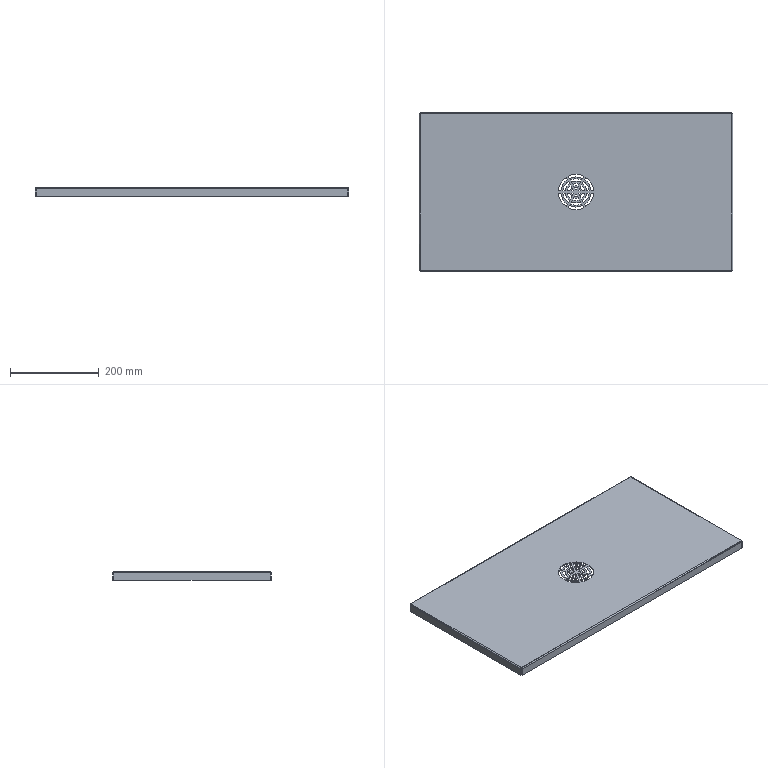Part | STEP file | Lower seal plate | 1 solid | 134 faces | box 708 x 358 x 20 mm | volume 574512 mm3 | plane 70 | cylinder 56 | spline 8 | commonest cylinder face diameters 12 x6 20 x6 28 x6 40 x6 48 x6 60 x6